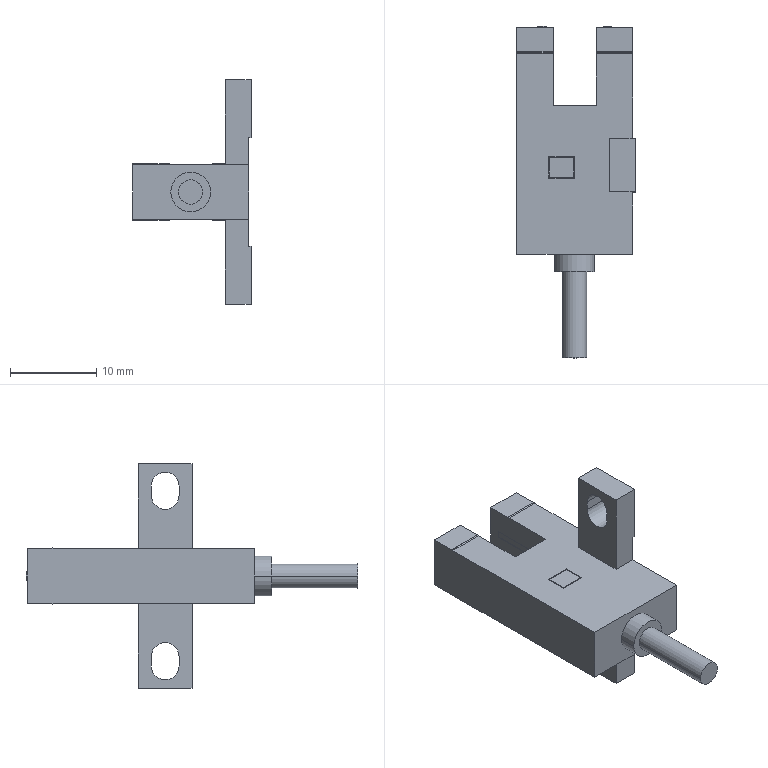Part | SolidWorks | features BaseBody 1 | 1 solid | 98 faces | box 13.7 x 38.4 x 26 mm | volume 2302 mm3 | plane 90 | cylinder 8 | commonest cylinder face diameters 3.2 x4 2.8 x2 4.6 x2